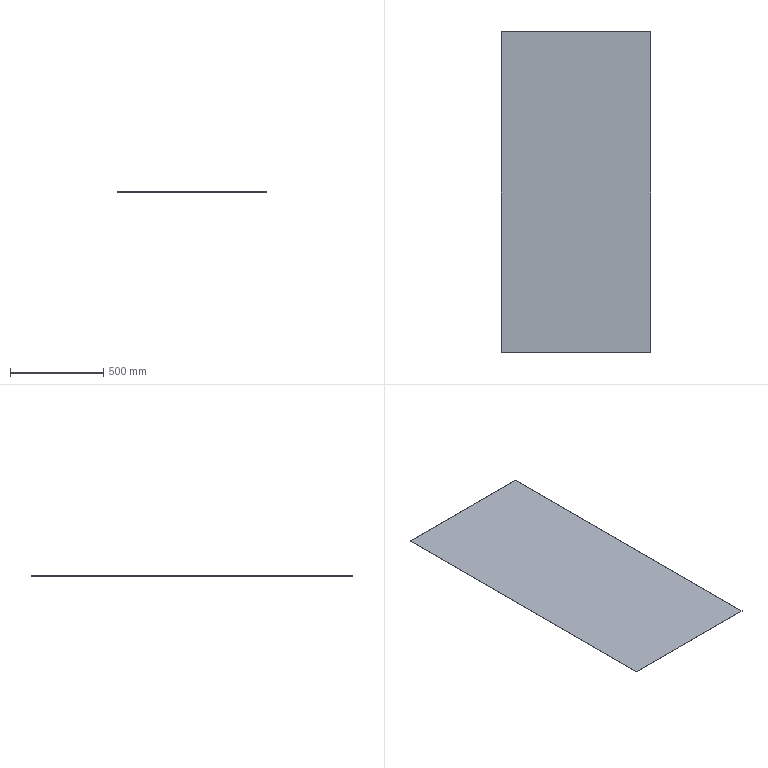Part | SolidWorks | features Extrusion 1 | 1 solid | 6 faces | box 800 x 1720 x 1 mm | volume 1376000 mm3 | plane 6
STEP:
#1=CARTESIAN_POINT('',(-400.,860.,0.));
#2=VERTEX_POINT('',#1);
#3=CARTESIAN_POINT('',(-400.,-860.,0.));
#4=VERTEX_POINT('',#3);
#5=CARTESIAN_POINT('',(-400.,-860.,0.));
#6=DIRECTION('',(0.,-1.,0.));
#7=VECTOR('',#6,1000.);
#8=LINE('',#5,#7);
#9=EDGE_CURVE('',#2,#4,#8,.T.);
#10=ORIENTED_EDGE('',*,*,#9,.T.);
#11=CARTESIAN_POINT('',(-400.,-860.,1.));
#12=VERTEX_POINT('',#11);
#13=CARTESIAN_POINT('',(-400.,-860.,1.));
#14=DIRECTION('',(0.,0.,-1.));
#15=VECTOR('',#14,1000.);
#16=LINE('',#13,#15);
#17=EDGE_CURVE('',#12,#4,#16,.T.);
#18=ORIENTED_EDGE('',*,*,#17,.F.);
#19=CARTESIAN_POINT('',(-400.,860.,1.));
#20=VERTEX_POINT('',#19);
#21=CARTESIAN_POINT('',(-400.,-860.,1.));
#22=DIRECTION('',(0.,-1.,0.));
#23=VECTOR('',#22,1000.);
#24=LINE('',#21,#23);
#25=EDGE_CURVE('',#20,#12,#24,.T.);
#26=ORIENTED_EDGE('',*,*,#25,.F.);
#27=CARTESIAN_POINT('',(-400.,860.,1.));
#28=DIRECTION('',(0.,0.,-1.));
#29=VECTOR('',#28,1000.);
#30=LINE('',#27,#29);
#31=EDGE_CURVE('',#20,#2,#30,.T.);
#32=ORIENTED_EDGE('',*,*,#31,.T.);
#33=EDGE_LOOP('',(#10,#18,#26,#32));
#34=FACE_OUTER_BOUND('',#33,.T.);
#35=CARTESIAN_POINT('',(-400.,-860.,1.));
#36=DIRECTION('',(1.,0.,0.));
#37=DIRECTION('',(0.,0.,-1.));
#38=AXIS2_PLACEMENT_3D('',#35,#36,#37);
#39=PLANE('',#38);
#40=ADVANCED_FACE('',(#34),#39,.F.);
#41=CARTESIAN_POINT('',(400.,-860.,0.));
#42=VERTEX_POINT('',#41);
#43=CARTESIAN_POINT('',(400.,-860.,0.));
#44=DIRECTION('',(1.,0.,0.));
#45=VECTOR('',#44,1000.);
#46=LINE('',#43,#45);
#47=EDGE_CURVE('',#4,#42,#46,.T.);
#48=ORIENTED_EDGE('',*,*,#47,.T.);
#49=CARTESIAN_POINT('',(400.,-860.,1.));
#50=VERTEX_POINT('',#49);
#51=CARTESIAN_POINT('',(400.,-860.,1.));
#52=DIRECTION('',(0.,0.,-1.));
#53=VECTOR('',#52,1000.);
#54=LINE('',#51,#53);
#55=EDGE_CURVE('',#50,#42,#54,.T.);
#56=ORIENTED_EDGE('',*,*,#55,.F.);
#57=CARTESIAN_POINT('',(400.,-860.,1.));
#58=DIRECTION('',(1.,0.,0.));
#59=VECTOR('',#58,1000.);
#60=LINE('',#57,#59);
#61=EDGE_CURVE('',#12,#50,#60,.T.);
#62=ORIENTED_EDGE('',*,*,#61,.F.);
#63=ORIENTED_EDGE('',*,*,#17,.T.);
#64=EDGE_LOOP('',(#48,#56,#62,#63));
#65=FACE_OUTER_BOUND('',#64,.T.);
#66=CARTESIAN_POINT('',(400.,-860.,1.));
#67=DIRECTION('',(0.,1.,0.));
#68=DIRECTION('',(-1.,0.,0.));
#69=AXIS2_PLACEMENT_3D('',#66,#67,#68);
#70=PLANE('',#69);
#71=ADVANCED_FACE('',(#65),#70,.F.);
#72=CARTESIAN_POINT('',(400.,860.,0.));
#73=VERTEX_POINT('',#72);
#74=CARTESIAN_POINT('',(400.,-860.,0.));
#75=DIRECTION('',(0.,1.,0.));
#76=VECTOR('',#75,1000.);
#77=LINE('',#74,#76);
#78=EDGE_CURVE('',#42,#73,#77,.T.);
#79=ORIENTED_EDGE('',*,*,#78,.T.);
#80=CARTESIAN_POINT('',(400.,860.,1.));
#81=VERTEX_POINT('',#80);
#82=CARTESIAN_POINT('',(400.,860.,1.));
#83=DIRECTION('',(0.,0.,-1.));
#84=VECTOR('',#83,1000.);
#85=LINE('',#82,#84);
#86=EDGE_CURVE('',#81,#73,#85,.T.);
#87=ORIENTED_EDGE('',*,*,#86,.F.);
#88=CARTESIAN_POINT('',(400.,-860.,1.));
#89=DIRECTION('',(0.,1.,0.));
#90=VECTOR('',#89,1000.);
#91=LINE('',#88,#90);
#92=EDGE_CURVE('',#50,#81,#91,.T.);
#93=ORIENTED_EDGE('',*,*,#92,.F.);
#94=ORIENTED_EDGE('',*,*,#55,.T.);
#95=EDGE_LOOP('',(#79,#87,#93,#94));
#96=FACE_OUTER_BOUND('',#95,.T.);
#97=CARTESIAN_POINT('',(400.,-860.,1.));
#98=DIRECTION('',(-1.,0.,0.));
#99=DIRECTION('',(0.,0.,1.));
#100=AXIS2_PLACEMENT_3D('',#97,#98,#99);
#101=PLANE('',#100);
#102=ADVANCED_FACE('',(#96),#101,.F.);
#103=CARTESIAN_POINT('',(400.,860.,0.));
#104=DIRECTION('',(-1.,0.,0.));
#105=VECTOR('',#104,1000.);
#106=LINE('',#103,#105);
#107=EDGE_CURVE('',#73,#2,#106,.T.);
#108=ORIENTED_EDGE('',*,*,#107,.T.);
#109=ORIENTED_EDGE('',*,*,#31,.F.);
#110=CARTESIAN_POINT('',(400.,860.,1.));
#111=DIRECTION('',(-1.,0.,0.));
#112=VECTOR('',#111,1000.);
#113=LINE('',#110,#112);
#114=EDGE_CURVE('',#81,#20,#113,.T.);
#115=ORIENTED_EDGE('',*,*,#114,.F.);
#116=ORIENTED_EDGE('',*,*,#86,.T.);
#117=EDGE_LOOP('',(#108,#109,#115,#116));
#118=FACE_OUTER_BOUND('',#117,.T.);
#119=CARTESIAN_POINT('',(400.,860.,1.));
#120=DIRECTION('',(0.,-1.,0.));
#121=DIRECTION('',(1.,0.,0.));
#122=AXIS2_PLACEMENT_3D('',#119,#120,#121);
#123=PLANE('',#122);
#124=ADVANCED_FACE('',(#118),#123,.F.);
#125=ORIENTED_EDGE('',*,*,#25,.T.);
#126=ORIENTED_EDGE('',*,*,#61,.T.);
#127=ORIENTED_EDGE('',*,*,#92,.T.);
#128=ORIENTED_EDGE('',*,*,#114,.T.);
#129=EDGE_LOOP('',(#125,#126,#127,#128));
#130=FACE_OUTER_BOUND('',#129,.T.);
#131=CARTESIAN_POINT('',(0.,0.,1.));
#132=DIRECTION('',(0.,0.,1.));
#133=DIRECTION('',(1.,0.,0.));
#134=AXIS2_PLACEMENT_3D('',#131,#132,#133);
#135=PLANE('',#134);
#136=ADVANCED_FACE('',(#130),#135,.T.);
#137=ORIENTED_EDGE('',*,*,#9,.F.);
#138=ORIENTED_EDGE('',*,*,#107,.F.);
#139=ORIENTED_EDGE('',*,*,#78,.F.);
#140=ORIENTED_EDGE('',*,*,#47,.F.);
#141=EDGE_LOOP('',(#137,#138,#139,#140));
#142=FACE_OUTER_BOUND('',#141,.T.);
#143=CARTESIAN_POINT('',(0.,0.,0.));
#144=DIRECTION('',(0.,0.,1.));
#145=DIRECTION('',(1.,0.,0.));
#146=AXIS2_PLACEMENT_3D('',#143,#144,#145);
#147=PLANE('',#146);
#148=ADVANCED_FACE('',(#142),#147,.F.);
#149=CLOSED_SHELL('',(#40,#71,#102,#124,#136,#148));
#150=MANIFOLD_SOLID_BREP('',#149);
#151=CARTESIAN_POINT('',(0.,0.,0.));
#152=DIRECTION('',(0.,0.,1.));
#153=DIRECTION('',(1.,0.,0.));
#154=AXIS2_PLACEMENT_3D('',#151,#152,#153);
#155=(LENGTH_UNIT()NAMED_UNIT(*)SI_UNIT(.MILLI.,.METRE.));
#156=UNCERTAINTY_MEASURE_WITH_UNIT(LENGTH_MEASURE(0.00001),#155,'','');
#157=(NAMED_UNIT(*)PLANE_ANGLE_UNIT()SI_UNIT($,.RADIAN.));
#158=(NAMED_UNIT(*)SI_UNIT($,.STERADIAN.)SOLID_ANGLE_UNIT());
#159=(GEOMETRIC_REPRESENTATION_CONTEXT(3)GLOBAL_UNCERTAINTY_ASSIGNED_CONTEXT((#156))GLOBAL_UNIT_ASSIGNED_CONTEXT((#155,#157,#158))REPRESENTATION_CONTEXT('',''));
#160=ADVANCED_BREP_SHAPE_REPRESENTATION('',(#150,#154),#159);